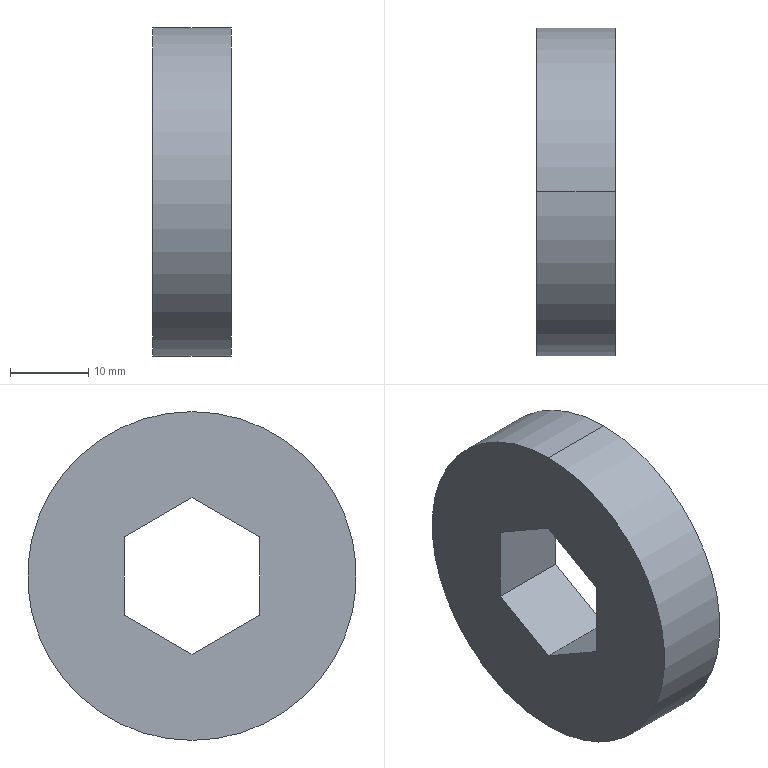Part | NX | 1 solid | 10 faces | box 10 x 42 x 42 mm | volume 11256 mm3 | plane 8 | cylinder 2 | commonest cylinder face diameters 42 x2
STEP:
#1=CARTESIAN_POINT('',(10.,0.,-21.));
#2=VERTEX_POINT('',#1);
#3=CARTESIAN_POINT('',(10.,0.,21.));
#4=VERTEX_POINT('',#3);
#5=CARTESIAN_POINT('',(10.,0.,0.));
#6=DIRECTION('',(1.,0.,0.));
#7=DIRECTION('',(0.,0.,-1.));
#8=AXIS2_PLACEMENT_3D('',#5,#6,#7);
#9=CIRCLE('',#8,21.);
#10=EDGE_CURVE('',#2,#4,#9,.T.);
#11=ORIENTED_EDGE('',*,*,#10,.F.);
#12=CARTESIAN_POINT('',(0.,0.,-21.));
#13=VERTEX_POINT('',#12);
#14=CARTESIAN_POINT('',(10.,0.,-21.));
#15=DIRECTION('',(-1.,0.,0.));
#16=VECTOR('',#15,1.);
#17=LINE('',#14,#16);
#18=EDGE_CURVE('',#2,#13,#17,.T.);
#19=ORIENTED_EDGE('',*,*,#18,.T.);
#20=CARTESIAN_POINT('',(0.,0.,21.));
#21=VERTEX_POINT('',#20);
#22=CARTESIAN_POINT('',(0.,0.,0.));
#23=DIRECTION('',(1.,0.,0.));
#24=DIRECTION('',(0.,0.,-1.));
#25=AXIS2_PLACEMENT_3D('',#22,#23,#24);
#26=CIRCLE('',#25,21.);
#27=EDGE_CURVE('',#13,#21,#26,.T.);
#28=ORIENTED_EDGE('',*,*,#27,.T.);
#29=CARTESIAN_POINT('',(10.,0.,21.));
#30=DIRECTION('',(-1.,0.,0.));
#31=VECTOR('',#30,1.);
#32=LINE('',#29,#31);
#33=EDGE_CURVE('',#4,#21,#32,.T.);
#34=ORIENTED_EDGE('',*,*,#33,.F.);
#35=EDGE_LOOP('',(#11,#19,#28,#34));
#36=FACE_OUTER_BOUND('',#35,.T.);
#37=CARTESIAN_POINT('',(10.,0.,0.));
#38=DIRECTION('',(-1.,0.,0.));
#39=DIRECTION('',(0.,0.,1.));
#40=AXIS2_PLACEMENT_3D('',#37,#38,#39);
#41=CYLINDRICAL_SURFACE('',#40,21.);
#42=ADVANCED_FACE('',(#36),#41,.T.);
#43=CARTESIAN_POINT('',(10.,0.,0.));
#44=DIRECTION('',(1.,0.,0.));
#45=DIRECTION('',(0.,0.,-1.));
#46=AXIS2_PLACEMENT_3D('',#43,#44,#45);
#47=CIRCLE('',#46,21.);
#48=EDGE_CURVE('',#4,#2,#47,.T.);
#49=ORIENTED_EDGE('',*,*,#48,.T.);
#50=ORIENTED_EDGE('',*,*,#10,.T.);
#51=EDGE_LOOP('',(#49,#50));
#52=FACE_BOUND('',#51,.T.);
#53=CARTESIAN_POINT('',(10.,0.,-10.));
#54=VERTEX_POINT('',#53);
#55=CARTESIAN_POINT('',(10.,8.66,-5.));
#56=VERTEX_POINT('',#55);
#57=CARTESIAN_POINT('',(10.,0.,-10.));
#58=DIRECTION('',(0.,0.866,0.5));
#59=VECTOR('',#58,1.);
#60=LINE('',#57,#59);
#61=EDGE_CURVE('',#54,#56,#60,.T.);
#62=ORIENTED_EDGE('',*,*,#61,.F.);
#63=CARTESIAN_POINT('',(10.,-8.66,-5.));
#64=VERTEX_POINT('',#63);
#65=CARTESIAN_POINT('',(10.,-8.66,-5.));
#66=DIRECTION('',(0.,0.866,-0.5));
#67=VECTOR('',#66,1.);
#68=LINE('',#65,#67);
#69=EDGE_CURVE('',#64,#54,#68,.T.);
#70=ORIENTED_EDGE('',*,*,#69,.F.);
#71=CARTESIAN_POINT('',(10.,-8.66,5.));
#72=VERTEX_POINT('',#71);
#73=CARTESIAN_POINT('',(10.,-8.66,5.));
#74=DIRECTION('',(0.,0.,-1.));
#75=VECTOR('',#74,1.);
#76=LINE('',#73,#75);
#77=EDGE_CURVE('',#72,#64,#76,.T.);
#78=ORIENTED_EDGE('',*,*,#77,.F.);
#79=CARTESIAN_POINT('',(10.,0.,10.));
#80=VERTEX_POINT('',#79);
#81=CARTESIAN_POINT('',(10.,0.,10.));
#82=DIRECTION('',(0.,-0.866,-0.5));
#83=VECTOR('',#82,1.);
#84=LINE('',#81,#83);
#85=EDGE_CURVE('',#80,#72,#84,.T.);
#86=ORIENTED_EDGE('',*,*,#85,.F.);
#87=CARTESIAN_POINT('',(10.,8.66,5.));
#88=VERTEX_POINT('',#87);
#89=CARTESIAN_POINT('',(10.,8.66,5.));
#90=DIRECTION('',(0.,-0.866,0.5));
#91=VECTOR('',#90,1.);
#92=LINE('',#89,#91);
#93=EDGE_CURVE('',#88,#80,#92,.T.);
#94=ORIENTED_EDGE('',*,*,#93,.F.);
#95=CARTESIAN_POINT('',(10.,8.66,-5.));
#96=DIRECTION('',(0.,0.,1.));
#97=VECTOR('',#96,1.);
#98=LINE('',#95,#97);
#99=EDGE_CURVE('',#56,#88,#98,.T.);
#100=ORIENTED_EDGE('',*,*,#99,.F.);
#101=EDGE_LOOP('',(#62,#70,#78,#86,#94,#100));
#102=FACE_BOUND('',#101,.T.);
#103=CARTESIAN_POINT('',(10.,0.,0.));
#104=DIRECTION('',(1.,0.,0.));
#105=DIRECTION('',(0.,0.,-1.));
#106=AXIS2_PLACEMENT_3D('',#103,#104,#105);
#107=PLANE('',#106);
#108=ADVANCED_FACE('',(#52,#102),#107,.T.);
#109=CARTESIAN_POINT('',(0.,0.,0.));
#110=DIRECTION('',(1.,0.,0.));
#111=DIRECTION('',(0.,0.,-1.));
#112=AXIS2_PLACEMENT_3D('',#109,#110,#111);
#113=CIRCLE('',#112,21.);
#114=EDGE_CURVE('',#21,#13,#113,.T.);
#115=ORIENTED_EDGE('',*,*,#114,.F.);
#116=ORIENTED_EDGE('',*,*,#27,.F.);
#117=EDGE_LOOP('',(#115,#116));
#118=FACE_BOUND('',#117,.T.);
#119=CARTESIAN_POINT('',(0.,-8.66,-5.));
#120=VERTEX_POINT('',#119);
#121=CARTESIAN_POINT('',(0.,0.,-10.));
#122=VERTEX_POINT('',#121);
#123=CARTESIAN_POINT('',(0.,-8.66,-5.));
#124=DIRECTION('',(0.,0.866,-0.5));
#125=VECTOR('',#124,1.);
#126=LINE('',#123,#125);
#127=EDGE_CURVE('',#120,#122,#126,.T.);
#128=ORIENTED_EDGE('',*,*,#127,.T.);
#129=CARTESIAN_POINT('',(0.,8.66,-5.));
#130=VERTEX_POINT('',#129);
#131=CARTESIAN_POINT('',(0.,0.,-10.));
#132=DIRECTION('',(0.,0.866,0.5));
#133=VECTOR('',#132,1.);
#134=LINE('',#131,#133);
#135=EDGE_CURVE('',#122,#130,#134,.T.);
#136=ORIENTED_EDGE('',*,*,#135,.T.);
#137=CARTESIAN_POINT('',(0.,8.66,5.));
#138=VERTEX_POINT('',#137);
#139=CARTESIAN_POINT('',(0.,8.66,-5.));
#140=DIRECTION('',(0.,0.,1.));
#141=VECTOR('',#140,1.);
#142=LINE('',#139,#141);
#143=EDGE_CURVE('',#130,#138,#142,.T.);
#144=ORIENTED_EDGE('',*,*,#143,.T.);
#145=CARTESIAN_POINT('',(0.,0.,10.));
#146=VERTEX_POINT('',#145);
#147=CARTESIAN_POINT('',(0.,8.66,5.));
#148=DIRECTION('',(0.,-0.866,0.5));
#149=VECTOR('',#148,1.);
#150=LINE('',#147,#149);
#151=EDGE_CURVE('',#138,#146,#150,.T.);
#152=ORIENTED_EDGE('',*,*,#151,.T.);
#153=CARTESIAN_POINT('',(0.,-8.66,5.));
#154=VERTEX_POINT('',#153);
#155=CARTESIAN_POINT('',(0.,0.,10.));
#156=DIRECTION('',(0.,-0.866,-0.5));
#157=VECTOR('',#156,1.);
#158=LINE('',#155,#157);
#159=EDGE_CURVE('',#146,#154,#158,.T.);
#160=ORIENTED_EDGE('',*,*,#159,.T.);
#161=CARTESIAN_POINT('',(0.,-8.66,5.));
#162=DIRECTION('',(0.,0.,-1.));
#163=VECTOR('',#162,1.);
#164=LINE('',#161,#163);
#165=EDGE_CURVE('',#154,#120,#164,.T.);
#166=ORIENTED_EDGE('',*,*,#165,.T.);
#167=EDGE_LOOP('',(#128,#136,#144,#152,#160,#166));
#168=FACE_BOUND('',#167,.T.);
#169=CARTESIAN_POINT('',(0.,0.,0.));
#170=DIRECTION('',(1.,0.,0.));
#171=DIRECTION('',(0.,0.,-1.));
#172=AXIS2_PLACEMENT_3D('',#169,#170,#171);
#173=PLANE('',#172);
#174=ADVANCED_FACE('',(#118,#168),#173,.F.);
#175=ORIENTED_EDGE('',*,*,#18,.F.);
#176=ORIENTED_EDGE('',*,*,#48,.F.);
#177=ORIENTED_EDGE('',*,*,#33,.T.);
#178=ORIENTED_EDGE('',*,*,#114,.T.);
#179=EDGE_LOOP('',(#175,#176,#177,#178));
#180=FACE_OUTER_BOUND('',#179,.T.);
#181=CARTESIAN_POINT('',(10.,0.,0.));
#182=DIRECTION('',(-1.,0.,0.));
#183=DIRECTION('',(0.,0.,1.));
#184=AXIS2_PLACEMENT_3D('',#181,#182,#183);
#185=CYLINDRICAL_SURFACE('',#184,21.);
#186=ADVANCED_FACE('',(#180),#185,.T.);
#187=ORIENTED_EDGE('',*,*,#127,.F.);
#188=CARTESIAN_POINT('',(10.,-8.66,-5.));
#189=DIRECTION('',(-1.,0.,0.));
#190=VECTOR('',#189,1.);
#191=LINE('',#188,#190);
#192=EDGE_CURVE('',#64,#120,#191,.T.);
#193=ORIENTED_EDGE('',*,*,#192,.F.);
#194=ORIENTED_EDGE('',*,*,#69,.T.);
#195=CARTESIAN_POINT('',(10.,0.,-10.));
#196=DIRECTION('',(-1.,0.,0.));
#197=VECTOR('',#196,1.);
#198=LINE('',#195,#197);
#199=EDGE_CURVE('',#54,#122,#198,.T.);
#200=ORIENTED_EDGE('',*,*,#199,.T.);
#201=EDGE_LOOP('',(#187,#193,#194,#200));
#202=FACE_OUTER_BOUND('',#201,.T.);
#203=CARTESIAN_POINT('',(10.,-8.66,-5.));
#204=DIRECTION('',(0.,0.5,0.866));
#205=DIRECTION('',(0.,-0.866,0.5));
#206=AXIS2_PLACEMENT_3D('',#203,#204,#205);
#207=PLANE('',#206);
#208=ADVANCED_FACE('',(#202),#207,.T.);
#209=ORIENTED_EDGE('',*,*,#135,.F.);
#210=ORIENTED_EDGE('',*,*,#199,.F.);
#211=ORIENTED_EDGE('',*,*,#61,.T.);
#212=CARTESIAN_POINT('',(10.,8.66,-5.));
#213=DIRECTION('',(-1.,0.,0.));
#214=VECTOR('',#213,1.);
#215=LINE('',#212,#214);
#216=EDGE_CURVE('',#56,#130,#215,.T.);
#217=ORIENTED_EDGE('',*,*,#216,.T.);
#218=EDGE_LOOP('',(#209,#210,#211,#217));
#219=FACE_OUTER_BOUND('',#218,.T.);
#220=CARTESIAN_POINT('',(10.,0.,-10.));
#221=DIRECTION('',(0.,-0.5,0.866));
#222=DIRECTION('',(0.,-0.866,-0.5));
#223=AXIS2_PLACEMENT_3D('',#220,#221,#222);
#224=PLANE('',#223);
#225=ADVANCED_FACE('',(#219),#224,.T.);
#226=ORIENTED_EDGE('',*,*,#143,.F.);
#227=ORIENTED_EDGE('',*,*,#216,.F.);
#228=ORIENTED_EDGE('',*,*,#99,.T.);
#229=CARTESIAN_POINT('',(10.,8.66,5.));
#230=DIRECTION('',(-1.,0.,0.));
#231=VECTOR('',#230,1.);
#232=LINE('',#229,#231);
#233=EDGE_CURVE('',#88,#138,#232,.T.);
#234=ORIENTED_EDGE('',*,*,#233,.T.);
#235=EDGE_LOOP('',(#226,#227,#228,#234));
#236=FACE_OUTER_BOUND('',#235,.T.);
#237=CARTESIAN_POINT('',(10.,8.66,-5.));
#238=DIRECTION('',(0.,-1.,0.));
#239=DIRECTION('',(0.,0.,-1.));
#240=AXIS2_PLACEMENT_3D('',#237,#238,#239);
#241=PLANE('',#240);
#242=ADVANCED_FACE('',(#236),#241,.T.);
#243=ORIENTED_EDGE('',*,*,#151,.F.);
#244=ORIENTED_EDGE('',*,*,#233,.F.);
#245=ORIENTED_EDGE('',*,*,#93,.T.);
#246=CARTESIAN_POINT('',(10.,0.,10.));
#247=DIRECTION('',(-1.,0.,0.));
#248=VECTOR('',#247,1.);
#249=LINE('',#246,#248);
#250=EDGE_CURVE('',#80,#146,#249,.T.);
#251=ORIENTED_EDGE('',*,*,#250,.T.);
#252=EDGE_LOOP('',(#243,#244,#245,#251));
#253=FACE_OUTER_BOUND('',#252,.T.);
#254=CARTESIAN_POINT('',(10.,8.66,5.));
#255=DIRECTION('',(0.,-0.5,-0.866));
#256=DIRECTION('',(0.,0.866,-0.5));
#257=AXIS2_PLACEMENT_3D('',#254,#255,#256);
#258=PLANE('',#257);
#259=ADVANCED_FACE('',(#253),#258,.T.);
#260=ORIENTED_EDGE('',*,*,#159,.F.);
#261=ORIENTED_EDGE('',*,*,#250,.F.);
#262=ORIENTED_EDGE('',*,*,#85,.T.);
#263=CARTESIAN_POINT('',(10.,-8.66,5.));
#264=DIRECTION('',(-1.,0.,0.));
#265=VECTOR('',#264,1.);
#266=LINE('',#263,#265);
#267=EDGE_CURVE('',#72,#154,#266,.T.);
#268=ORIENTED_EDGE('',*,*,#267,.T.);
#269=EDGE_LOOP('',(#260,#261,#262,#268));
#270=FACE_OUTER_BOUND('',#269,.T.);
#271=CARTESIAN_POINT('',(10.,0.,10.));
#272=DIRECTION('',(0.,0.5,-0.866));
#273=DIRECTION('',(0.,0.866,0.5));
#274=AXIS2_PLACEMENT_3D('',#271,#272,#273);
#275=PLANE('',#274);
#276=ADVANCED_FACE('',(#270),#275,.T.);
#277=ORIENTED_EDGE('',*,*,#165,.F.);
#278=ORIENTED_EDGE('',*,*,#267,.F.);
#279=ORIENTED_EDGE('',*,*,#77,.T.);
#280=ORIENTED_EDGE('',*,*,#192,.T.);
#281=EDGE_LOOP('',(#277,#278,#279,#280));
#282=FACE_OUTER_BOUND('',#281,.T.);
#283=CARTESIAN_POINT('',(10.,-8.66,5.));
#284=DIRECTION('',(0.,1.,0.));
#285=DIRECTION('',(0.,0.,1.));
#286=AXIS2_PLACEMENT_3D('',#283,#284,#285);
#287=PLANE('',#286);
#288=ADVANCED_FACE('',(#282),#287,.T.);
#289=CLOSED_SHELL('',(#42,#108,#174,#186,#208,#225,#242,#259,#276,#288));
#290=MANIFOLD_SOLID_BREP('',#289);
#291=(LENGTH_UNIT()NAMED_UNIT(*)SI_UNIT(.MILLI.,.METRE.));
#292=UNCERTAINTY_MEASURE_WITH_UNIT(LENGTH_MEASURE(0.00002),#291,'','');
#293=(NAMED_UNIT(*)PLANE_ANGLE_UNIT()SI_UNIT($,.RADIAN.));
#294=PLANE_ANGLE_MEASURE_WITH_UNIT(PLANE_ANGLE_MEASURE(0.01745),#293);
#295=DIMENSIONAL_EXPONENTS(0.,0.,0.,0.,0.,0.,0.);
#296=(CONVERSION_BASED_UNIT('DEGREE',#294)NAMED_UNIT(#295)PLANE_ANGLE_UNIT());
#297=(NAMED_UNIT(*)SI_UNIT($,.STERADIAN.)SOLID_ANGLE_UNIT());
#298=(GEOMETRIC_REPRESENTATION_CONTEXT(3)GLOBAL_UNCERTAINTY_ASSIGNED_CONTEXT((#292))GLOBAL_UNIT_ASSIGNED_CONTEXT((#291,#296,#297))REPRESENTATION_CONTEXT('',''));
#299=ADVANCED_BREP_SHAPE_REPRESENTATION('',(#290),#298);